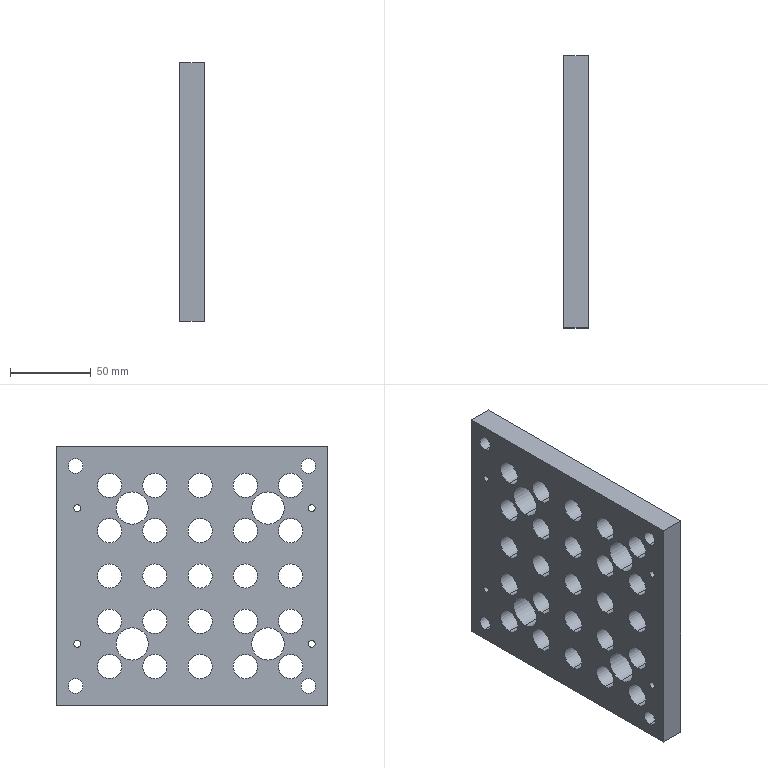Part | STEP file | 03-12 Battery stop plate | 1 solid | 80 faces | box 15 x 168 x 160 mm | volume 313434 mm3 | cylinder 74 | plane 6 | commonest cylinder face diameters 15 x50 4.2 x8 9 x8 20 x8